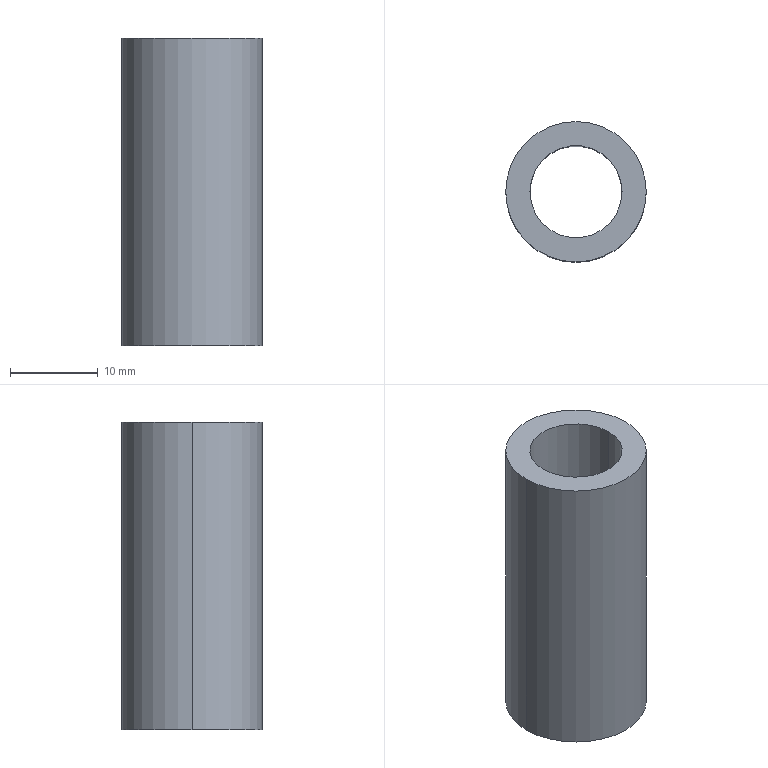Part | SolidWorks | features Extrusion 1, HoleWzd 1 | 1 solid | 6 faces | box 16 x 16 x 35 mm | volume 4007 mm3 | cylinder 4 | plane 2 | commonest cylinder face diameters 10.5 x2 16 x2
STEP:
#1=CARTESIAN_POINT('',(-5.25,0.,0.));
#2=VERTEX_POINT('',#1);
#3=CARTESIAN_POINT('',(5.25,0.,0.));
#4=VERTEX_POINT('',#3);
#5=CARTESIAN_POINT('',(0.,0.,0.));
#6=DIRECTION('',(0.,0.,1.));
#7=DIRECTION('',(1.,0.,0.));
#8=AXIS2_PLACEMENT_3D('',#5,#6,#7);
#9=CIRCLE('',#8,5.25);
#10=EDGE_CURVE('',#2,#4,#9,.T.);
#11=ORIENTED_EDGE('',*,*,#10,.F.);
#12=CARTESIAN_POINT('',(-5.25,0.,35.));
#13=VERTEX_POINT('',#12);
#14=CARTESIAN_POINT('',(-5.25,0.,35.));
#15=DIRECTION('',(0.,0.,1.));
#16=VECTOR('',#15,1000.);
#17=LINE('',#14,#16);
#18=EDGE_CURVE('',#2,#13,#17,.T.);
#19=ORIENTED_EDGE('',*,*,#18,.T.);
#20=CARTESIAN_POINT('',(5.25,0.,35.));
#21=VERTEX_POINT('',#20);
#22=CARTESIAN_POINT('',(0.,0.,35.));
#23=DIRECTION('',(0.,0.,1.));
#24=DIRECTION('',(1.,0.,0.));
#25=AXIS2_PLACEMENT_3D('',#22,#23,#24);
#26=CIRCLE('',#25,5.25);
#27=EDGE_CURVE('',#13,#21,#26,.T.);
#28=ORIENTED_EDGE('',*,*,#27,.T.);
#29=CARTESIAN_POINT('',(5.25,0.,35.));
#30=DIRECTION('',(0.,0.,1.));
#31=VECTOR('',#30,1000.);
#32=LINE('',#29,#31);
#33=EDGE_CURVE('',#4,#21,#32,.T.);
#34=ORIENTED_EDGE('',*,*,#33,.F.);
#35=EDGE_LOOP('',(#11,#19,#28,#34));
#36=FACE_OUTER_BOUND('',#35,.T.);
#37=CARTESIAN_POINT('',(0.,0.,35.));
#38=DIRECTION('',(0.,0.,1.));
#39=DIRECTION('',(1.,0.,0.));
#40=AXIS2_PLACEMENT_3D('',#37,#38,#39);
#41=CYLINDRICAL_SURFACE('',#40,5.25);
#42=ADVANCED_FACE('',(#36),#41,.F.);
#43=CARTESIAN_POINT('',(8.,0.,35.));
#44=VERTEX_POINT('',#43);
#45=CARTESIAN_POINT('',(-8.,0.,35.));
#46=VERTEX_POINT('',#45);
#47=CARTESIAN_POINT('',(0.,0.,35.));
#48=DIRECTION('',(0.,0.,1.));
#49=DIRECTION('',(1.,0.,0.));
#50=AXIS2_PLACEMENT_3D('',#47,#48,#49);
#51=CIRCLE('',#50,8.);
#52=EDGE_CURVE('',#44,#46,#51,.T.);
#53=ORIENTED_EDGE('',*,*,#52,.F.);
#54=CARTESIAN_POINT('',(8.,0.,0.));
#55=VERTEX_POINT('',#54);
#56=CARTESIAN_POINT('',(8.,0.,35.));
#57=DIRECTION('',(0.,0.,-1.));
#58=VECTOR('',#57,1000.);
#59=LINE('',#56,#58);
#60=EDGE_CURVE('',#44,#55,#59,.T.);
#61=ORIENTED_EDGE('',*,*,#60,.T.);
#62=CARTESIAN_POINT('',(-8.,0.,0.));
#63=VERTEX_POINT('',#62);
#64=CARTESIAN_POINT('',(0.,0.,0.));
#65=DIRECTION('',(0.,0.,1.));
#66=DIRECTION('',(1.,0.,0.));
#67=AXIS2_PLACEMENT_3D('',#64,#65,#66);
#68=CIRCLE('',#67,8.);
#69=EDGE_CURVE('',#55,#63,#68,.T.);
#70=ORIENTED_EDGE('',*,*,#69,.T.);
#71=CARTESIAN_POINT('',(-8.,0.,35.));
#72=DIRECTION('',(0.,0.,-1.));
#73=VECTOR('',#72,1000.);
#74=LINE('',#71,#73);
#75=EDGE_CURVE('',#46,#63,#74,.T.);
#76=ORIENTED_EDGE('',*,*,#75,.F.);
#77=EDGE_LOOP('',(#53,#61,#70,#76));
#78=FACE_OUTER_BOUND('',#77,.T.);
#79=CARTESIAN_POINT('',(0.,0.,35.));
#80=DIRECTION('',(0.,0.,-1.));
#81=DIRECTION('',(-1.,0.,0.));
#82=AXIS2_PLACEMENT_3D('',#79,#80,#81);
#83=CYLINDRICAL_SURFACE('',#82,8.);
#84=ADVANCED_FACE('',(#78),#83,.T.);
#85=ORIENTED_EDGE('',*,*,#60,.F.);
#86=CARTESIAN_POINT('',(0.,0.,35.));
#87=DIRECTION('',(0.,0.,1.));
#88=DIRECTION('',(1.,0.,0.));
#89=AXIS2_PLACEMENT_3D('',#86,#87,#88);
#90=CIRCLE('',#89,8.);
#91=EDGE_CURVE('',#46,#44,#90,.T.);
#92=ORIENTED_EDGE('',*,*,#91,.F.);
#93=ORIENTED_EDGE('',*,*,#75,.T.);
#94=CARTESIAN_POINT('',(0.,0.,0.));
#95=DIRECTION('',(0.,0.,1.));
#96=DIRECTION('',(1.,0.,0.));
#97=AXIS2_PLACEMENT_3D('',#94,#95,#96);
#98=CIRCLE('',#97,8.);
#99=EDGE_CURVE('',#63,#55,#98,.T.);
#100=ORIENTED_EDGE('',*,*,#99,.T.);
#101=EDGE_LOOP('',(#85,#92,#93,#100));
#102=FACE_OUTER_BOUND('',#101,.T.);
#103=CARTESIAN_POINT('',(0.,0.,35.));
#104=DIRECTION('',(0.,0.,-1.));
#105=DIRECTION('',(-1.,0.,0.));
#106=AXIS2_PLACEMENT_3D('',#103,#104,#105);
#107=CYLINDRICAL_SURFACE('',#106,8.);
#108=ADVANCED_FACE('',(#102),#107,.T.);
#109=CARTESIAN_POINT('',(0.,0.,35.));
#110=DIRECTION('',(0.,0.,1.));
#111=DIRECTION('',(1.,0.,0.));
#112=AXIS2_PLACEMENT_3D('',#109,#110,#111);
#113=CIRCLE('',#112,5.25);
#114=EDGE_CURVE('',#21,#13,#113,.T.);
#115=ORIENTED_EDGE('',*,*,#114,.F.);
#116=ORIENTED_EDGE('',*,*,#27,.F.);
#117=EDGE_LOOP('',(#115,#116));
#118=FACE_BOUND('',#117,.T.);
#119=ORIENTED_EDGE('',*,*,#91,.T.);
#120=ORIENTED_EDGE('',*,*,#52,.T.);
#121=EDGE_LOOP('',(#119,#120));
#122=FACE_OUTER_BOUND('',#121,.T.);
#123=CARTESIAN_POINT('',(0.,0.,35.));
#124=DIRECTION('',(0.,0.,1.));
#125=DIRECTION('',(1.,0.,0.));
#126=AXIS2_PLACEMENT_3D('',#123,#124,#125);
#127=PLANE('',#126);
#128=ADVANCED_FACE('',(#118,#122),#127,.T.);
#129=CARTESIAN_POINT('',(0.,0.,0.));
#130=DIRECTION('',(0.,0.,1.));
#131=DIRECTION('',(1.,0.,0.));
#132=AXIS2_PLACEMENT_3D('',#129,#130,#131);
#133=CIRCLE('',#132,5.25);
#134=EDGE_CURVE('',#4,#2,#133,.T.);
#135=ORIENTED_EDGE('',*,*,#134,.T.);
#136=ORIENTED_EDGE('',*,*,#10,.T.);
#137=EDGE_LOOP('',(#135,#136));
#138=FACE_BOUND('',#137,.T.);
#139=ORIENTED_EDGE('',*,*,#99,.F.);
#140=ORIENTED_EDGE('',*,*,#69,.F.);
#141=EDGE_LOOP('',(#139,#140));
#142=FACE_OUTER_BOUND('',#141,.T.);
#143=CARTESIAN_POINT('',(0.,0.,0.));
#144=DIRECTION('',(0.,0.,1.));
#145=DIRECTION('',(1.,0.,0.));
#146=AXIS2_PLACEMENT_3D('',#143,#144,#145);
#147=PLANE('',#146);
#148=ADVANCED_FACE('',(#138,#142),#147,.F.);
#149=ORIENTED_EDGE('',*,*,#18,.F.);
#150=ORIENTED_EDGE('',*,*,#134,.F.);
#151=ORIENTED_EDGE('',*,*,#33,.T.);
#152=ORIENTED_EDGE('',*,*,#114,.T.);
#153=EDGE_LOOP('',(#149,#150,#151,#152));
#154=FACE_OUTER_BOUND('',#153,.T.);
#155=CARTESIAN_POINT('',(0.,0.,35.));
#156=DIRECTION('',(0.,0.,1.));
#157=DIRECTION('',(1.,0.,0.));
#158=AXIS2_PLACEMENT_3D('',#155,#156,#157);
#159=CYLINDRICAL_SURFACE('',#158,5.25);
#160=ADVANCED_FACE('',(#154),#159,.F.);
#161=CLOSED_SHELL('',(#42,#84,#108,#128,#148,#160));
#162=MANIFOLD_SOLID_BREP('',#161);
#163=CARTESIAN_POINT('',(0.,0.,0.));
#164=DIRECTION('',(0.,0.,1.));
#165=DIRECTION('',(1.,0.,0.));
#166=AXIS2_PLACEMENT_3D('',#163,#164,#165);
#167=(LENGTH_UNIT()NAMED_UNIT(*)SI_UNIT(.MILLI.,.METRE.));
#168=UNCERTAINTY_MEASURE_WITH_UNIT(LENGTH_MEASURE(0.00001),#167,'','');
#169=(NAMED_UNIT(*)PLANE_ANGLE_UNIT()SI_UNIT($,.RADIAN.));
#170=(NAMED_UNIT(*)SI_UNIT($,.STERADIAN.)SOLID_ANGLE_UNIT());
#171=(GEOMETRIC_REPRESENTATION_CONTEXT(3)GLOBAL_UNCERTAINTY_ASSIGNED_CONTEXT((#168))GLOBAL_UNIT_ASSIGNED_CONTEXT((#167,#169,#170))REPRESENTATION_CONTEXT('',''));
#172=ADVANCED_BREP_SHAPE_REPRESENTATION('',(#162,#166),#171);